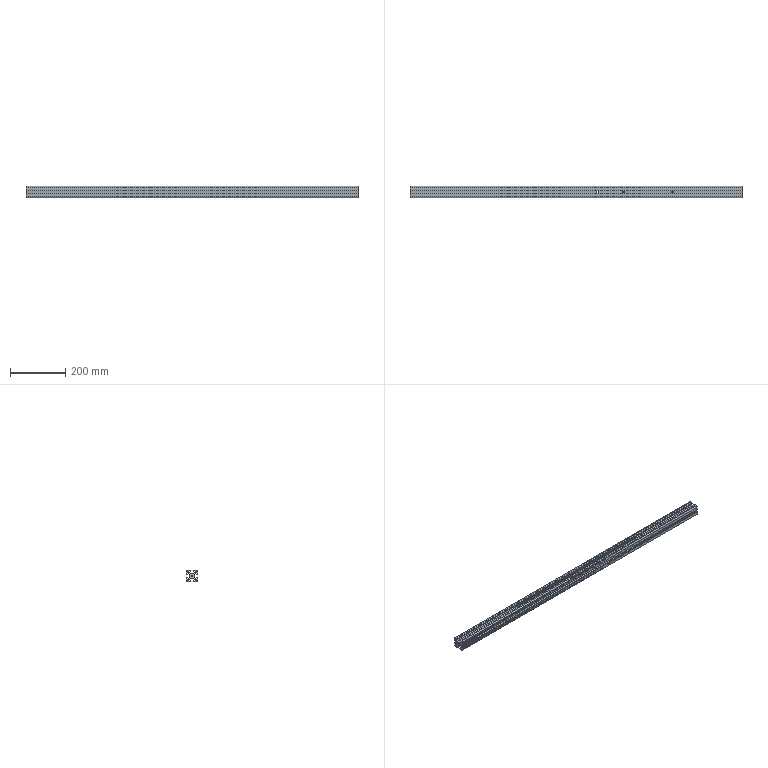Part | 1 solid | 116 faces | box 1200 x 40 x 40 mm | volume 690223 mm3 | plane 94 | cylinder 22 | commonest cylinder face diameters 6.8 x8 8.2 x6 5 x4 9 x4